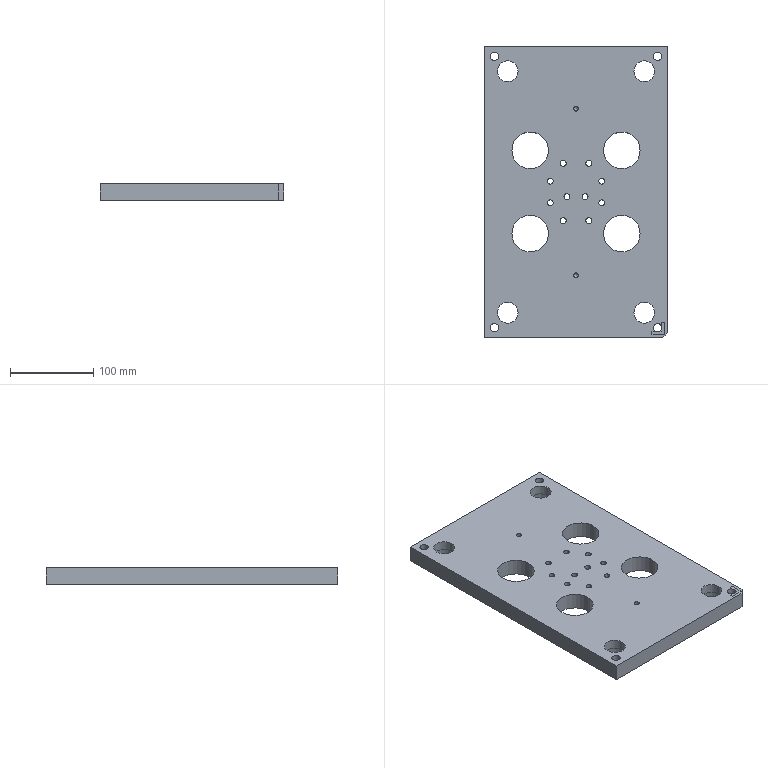Part | NX | features DZMB 2 | 1 solid | 75 faces | box 220 x 350 x 20 mm | volume 1351423 mm3 | cylinder 40 | plane 33 | cone 2 | commonest cylinder face diameters 7 x10 11 x10 10 x4 25 x4 31 x4 44 x4